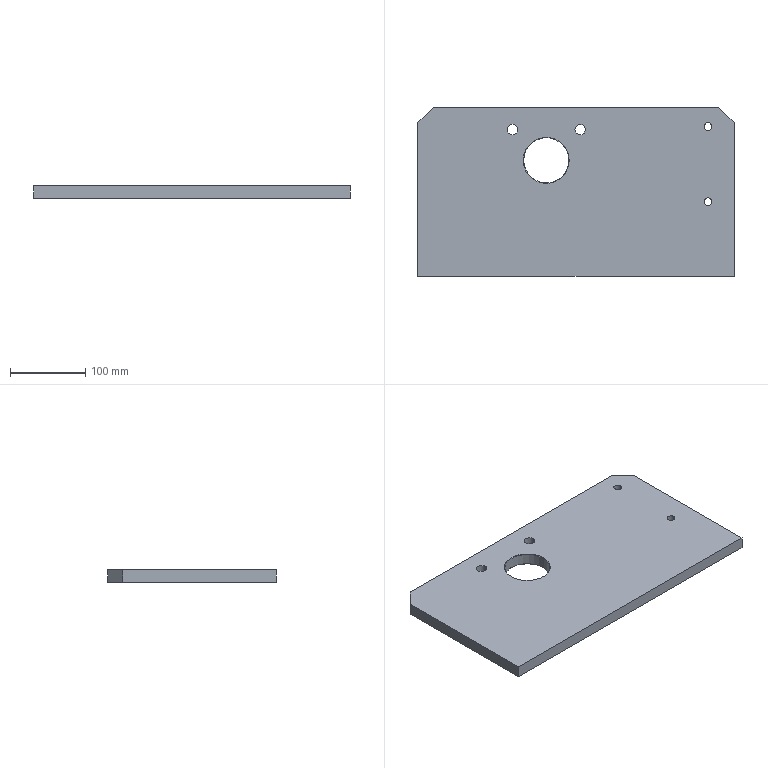Part | STEP file | 03-Vertical plate 1 | 1 solid | 22 faces | box 420 x 224 x 16 mm | volume 1446053 mm3 | cylinder 10 | plane 8 | cone 4 | commonest cylinder face diameters 10.2 x4 14 x4 60 x2